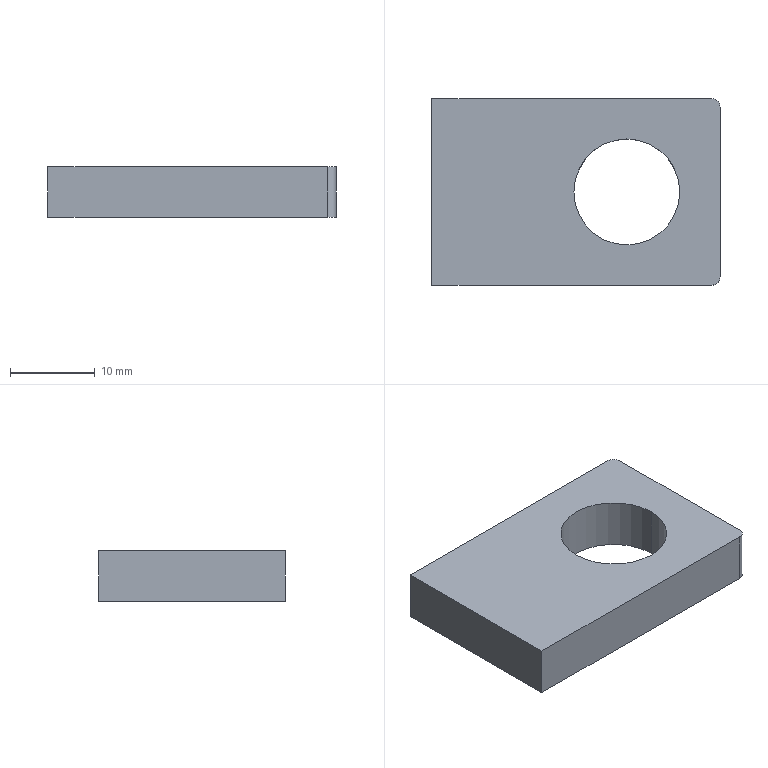Part | SolidWorks | features FlatPattern 1, SMBaseFlange 1, SheetMetal 1 | 1 solid | 10 faces | box 34 x 22 x 6 mm | volume 3749 mm3 | plane 6 | cylinder 4 | commonest cylinder face diameters 2 x2 12.5 x2
STEP:
#1=CARTESIAN_POINT('',(-6.25,0.,6.));
#2=VERTEX_POINT('',#1);
#3=CARTESIAN_POINT('',(6.25,0.,6.));
#4=VERTEX_POINT('',#3);
#5=CARTESIAN_POINT('',(0.,0.,6.));
#6=DIRECTION('',(0.,0.,1.));
#7=DIRECTION('',(1.,0.,0.));
#8=AXIS2_PLACEMENT_3D('',#5,#6,#7);
#9=CIRCLE('',#8,6.25);
#10=EDGE_CURVE('',#2,#4,#9,.T.);
#11=ORIENTED_EDGE('',*,*,#10,.T.);
#12=CARTESIAN_POINT('',(6.25,0.,0.));
#13=VERTEX_POINT('',#12);
#14=CARTESIAN_POINT('',(6.25,0.,6.));
#15=DIRECTION('',(0.,0.,-1.));
#16=VECTOR('',#15,1000.);
#17=LINE('',#14,#16);
#18=EDGE_CURVE('',#4,#13,#17,.T.);
#19=ORIENTED_EDGE('',*,*,#18,.T.);
#20=CARTESIAN_POINT('',(-6.25,0.,0.));
#21=VERTEX_POINT('',#20);
#22=CARTESIAN_POINT('',(0.,0.,0.));
#23=DIRECTION('',(0.,0.,1.));
#24=DIRECTION('',(1.,0.,0.));
#25=AXIS2_PLACEMENT_3D('',#22,#23,#24);
#26=CIRCLE('',#25,6.25);
#27=EDGE_CURVE('',#21,#13,#26,.T.);
#28=ORIENTED_EDGE('',*,*,#27,.F.);
#29=CARTESIAN_POINT('',(-6.25,0.,6.));
#30=DIRECTION('',(0.,0.,-1.));
#31=VECTOR('',#30,1000.);
#32=LINE('',#29,#31);
#33=EDGE_CURVE('',#2,#21,#32,.T.);
#34=ORIENTED_EDGE('',*,*,#33,.F.);
#35=EDGE_LOOP('',(#11,#19,#28,#34));
#36=FACE_OUTER_BOUND('',#35,.T.);
#37=CARTESIAN_POINT('',(0.,0.,6.));
#38=DIRECTION('',(0.,0.,-1.));
#39=DIRECTION('',(-1.,0.,0.));
#40=AXIS2_PLACEMENT_3D('',#37,#38,#39);
#41=CYLINDRICAL_SURFACE('',#40,6.25);
#42=ADVANCED_FACE('',(#36),#41,.F.);
#43=CARTESIAN_POINT('',(-23.,11.,6.));
#44=VERTEX_POINT('',#43);
#45=CARTESIAN_POINT('',(-23.,-11.,6.));
#46=VERTEX_POINT('',#45);
#47=CARTESIAN_POINT('',(-23.,11.,6.));
#48=DIRECTION('',(0.,-1.,0.));
#49=VECTOR('',#48,1000.);
#50=LINE('',#47,#49);
#51=EDGE_CURVE('',#44,#46,#50,.T.);
#52=ORIENTED_EDGE('',*,*,#51,.T.);
#53=CARTESIAN_POINT('',(10.,-11.,6.));
#54=VERTEX_POINT('',#53);
#55=CARTESIAN_POINT('',(10.,-11.,6.));
#56=DIRECTION('',(1.,0.,0.));
#57=VECTOR('',#56,1000.);
#58=LINE('',#55,#57);
#59=EDGE_CURVE('',#46,#54,#58,.T.);
#60=ORIENTED_EDGE('',*,*,#59,.T.);
#61=CARTESIAN_POINT('',(11.,-10.,6.));
#62=VERTEX_POINT('',#61);
#63=CARTESIAN_POINT('',(10.,-10.,6.));
#64=DIRECTION('',(0.,0.,1.));
#65=DIRECTION('',(-1.,0.,0.));
#66=AXIS2_PLACEMENT_3D('',#63,#64,#65);
#67=CIRCLE('',#66,1.);
#68=EDGE_CURVE('',#54,#62,#67,.T.);
#69=ORIENTED_EDGE('',*,*,#68,.T.);
#70=CARTESIAN_POINT('',(11.,10.,6.));
#71=VERTEX_POINT('',#70);
#72=CARTESIAN_POINT('',(11.,10.,6.));
#73=DIRECTION('',(0.,1.,0.));
#74=VECTOR('',#73,1000.);
#75=LINE('',#72,#74);
#76=EDGE_CURVE('',#62,#71,#75,.T.);
#77=ORIENTED_EDGE('',*,*,#76,.T.);
#78=CARTESIAN_POINT('',(10.,11.,6.));
#79=VERTEX_POINT('',#78);
#80=CARTESIAN_POINT('',(10.,10.,6.));
#81=DIRECTION('',(0.,0.,1.));
#82=DIRECTION('',(-1.,0.,0.));
#83=AXIS2_PLACEMENT_3D('',#80,#81,#82);
#84=CIRCLE('',#83,1.);
#85=EDGE_CURVE('',#71,#79,#84,.T.);
#86=ORIENTED_EDGE('',*,*,#85,.T.);
#87=CARTESIAN_POINT('',(10.,11.,6.));
#88=DIRECTION('',(-1.,0.,0.));
#89=VECTOR('',#88,1000.);
#90=LINE('',#87,#89);
#91=EDGE_CURVE('',#79,#44,#90,.T.);
#92=ORIENTED_EDGE('',*,*,#91,.T.);
#93=EDGE_LOOP('',(#52,#60,#69,#77,#86,#92));
#94=FACE_OUTER_BOUND('',#93,.T.);
#95=ORIENTED_EDGE('',*,*,#10,.F.);
#96=CARTESIAN_POINT('',(0.,0.,6.));
#97=DIRECTION('',(0.,0.,1.));
#98=DIRECTION('',(1.,0.,0.));
#99=AXIS2_PLACEMENT_3D('',#96,#97,#98);
#100=CIRCLE('',#99,6.25);
#101=EDGE_CURVE('',#4,#2,#100,.T.);
#102=ORIENTED_EDGE('',*,*,#101,.F.);
#103=EDGE_LOOP('',(#95,#102));
#104=FACE_BOUND('',#103,.T.);
#105=CARTESIAN_POINT('',(10.,-10.,6.));
#106=DIRECTION('',(0.,0.,-1.));
#107=DIRECTION('',(-1.,0.,0.));
#108=AXIS2_PLACEMENT_3D('',#105,#106,#107);
#109=PLANE('',#108);
#110=ADVANCED_FACE('',(#94,#104),#109,.F.);
#111=CARTESIAN_POINT('',(-23.,11.,0.));
#112=VERTEX_POINT('',#111);
#113=CARTESIAN_POINT('',(-23.,-11.,0.));
#114=VERTEX_POINT('',#113);
#115=CARTESIAN_POINT('',(-23.,11.,0.));
#116=DIRECTION('',(0.,-1.,0.));
#117=VECTOR('',#116,1000.);
#118=LINE('',#115,#117);
#119=EDGE_CURVE('',#112,#114,#118,.T.);
#120=ORIENTED_EDGE('',*,*,#119,.F.);
#121=CARTESIAN_POINT('',(10.,11.,0.));
#122=VERTEX_POINT('',#121);
#123=CARTESIAN_POINT('',(10.,11.,0.));
#124=DIRECTION('',(-1.,0.,0.));
#125=VECTOR('',#124,1000.);
#126=LINE('',#123,#125);
#127=EDGE_CURVE('',#122,#112,#126,.T.);
#128=ORIENTED_EDGE('',*,*,#127,.F.);
#129=CARTESIAN_POINT('',(11.,10.,0.));
#130=VERTEX_POINT('',#129);
#131=CARTESIAN_POINT('',(10.,10.,0.));
#132=DIRECTION('',(0.,0.,1.));
#133=DIRECTION('',(-1.,0.,0.));
#134=AXIS2_PLACEMENT_3D('',#131,#132,#133);
#135=CIRCLE('',#134,1.);
#136=EDGE_CURVE('',#130,#122,#135,.T.);
#137=ORIENTED_EDGE('',*,*,#136,.F.);
#138=CARTESIAN_POINT('',(11.,-10.,0.));
#139=VERTEX_POINT('',#138);
#140=CARTESIAN_POINT('',(11.,10.,0.));
#141=DIRECTION('',(0.,1.,0.));
#142=VECTOR('',#141,1000.);
#143=LINE('',#140,#142);
#144=EDGE_CURVE('',#139,#130,#143,.T.);
#145=ORIENTED_EDGE('',*,*,#144,.F.);
#146=CARTESIAN_POINT('',(10.,-11.,0.));
#147=VERTEX_POINT('',#146);
#148=CARTESIAN_POINT('',(10.,-10.,0.));
#149=DIRECTION('',(0.,0.,1.));
#150=DIRECTION('',(-1.,0.,0.));
#151=AXIS2_PLACEMENT_3D('',#148,#149,#150);
#152=CIRCLE('',#151,1.);
#153=EDGE_CURVE('',#147,#139,#152,.T.);
#154=ORIENTED_EDGE('',*,*,#153,.F.);
#155=CARTESIAN_POINT('',(10.,-11.,0.));
#156=DIRECTION('',(1.,0.,0.));
#157=VECTOR('',#156,1000.);
#158=LINE('',#155,#157);
#159=EDGE_CURVE('',#114,#147,#158,.T.);
#160=ORIENTED_EDGE('',*,*,#159,.F.);
#161=EDGE_LOOP('',(#120,#128,#137,#145,#154,#160));
#162=FACE_OUTER_BOUND('',#161,.T.);
#163=ORIENTED_EDGE('',*,*,#27,.T.);
#164=CARTESIAN_POINT('',(0.,0.,0.));
#165=DIRECTION('',(0.,0.,1.));
#166=DIRECTION('',(1.,0.,0.));
#167=AXIS2_PLACEMENT_3D('',#164,#165,#166);
#168=CIRCLE('',#167,6.25);
#169=EDGE_CURVE('',#13,#21,#168,.T.);
#170=ORIENTED_EDGE('',*,*,#169,.T.);
#171=EDGE_LOOP('',(#163,#170));
#172=FACE_BOUND('',#171,.T.);
#173=CARTESIAN_POINT('',(10.,-10.,0.));
#174=DIRECTION('',(0.,0.,-1.));
#175=DIRECTION('',(-1.,0.,0.));
#176=AXIS2_PLACEMENT_3D('',#173,#174,#175);
#177=PLANE('',#176);
#178=ADVANCED_FACE('',(#162,#172),#177,.T.);
#179=ORIENTED_EDGE('',*,*,#119,.T.);
#180=CARTESIAN_POINT('',(-23.,-11.,6.));
#181=DIRECTION('',(0.,0.,-1.));
#182=VECTOR('',#181,1000.);
#183=LINE('',#180,#182);
#184=EDGE_CURVE('',#46,#114,#183,.T.);
#185=ORIENTED_EDGE('',*,*,#184,.F.);
#186=ORIENTED_EDGE('',*,*,#51,.F.);
#187=CARTESIAN_POINT('',(-23.,11.,6.));
#188=DIRECTION('',(0.,0.,-1.));
#189=VECTOR('',#188,1000.);
#190=LINE('',#187,#189);
#191=EDGE_CURVE('',#44,#112,#190,.T.);
#192=ORIENTED_EDGE('',*,*,#191,.T.);
#193=EDGE_LOOP('',(#179,#185,#186,#192));
#194=FACE_OUTER_BOUND('',#193,.T.);
#195=CARTESIAN_POINT('',(-23.,11.,6.));
#196=DIRECTION('',(1.,0.,0.));
#197=DIRECTION('',(0.,1.,0.));
#198=AXIS2_PLACEMENT_3D('',#195,#196,#197);
#199=PLANE('',#198);
#200=ADVANCED_FACE('',(#194),#199,.F.);
#201=ORIENTED_EDGE('',*,*,#159,.T.);
#202=CARTESIAN_POINT('',(10.,-11.,6.));
#203=DIRECTION('',(0.,0.,-1.));
#204=VECTOR('',#203,1000.);
#205=LINE('',#202,#204);
#206=EDGE_CURVE('',#54,#147,#205,.T.);
#207=ORIENTED_EDGE('',*,*,#206,.F.);
#208=ORIENTED_EDGE('',*,*,#59,.F.);
#209=ORIENTED_EDGE('',*,*,#184,.T.);
#210=EDGE_LOOP('',(#201,#207,#208,#209));
#211=FACE_OUTER_BOUND('',#210,.T.);
#212=CARTESIAN_POINT('',(10.,-11.,6.));
#213=DIRECTION('',(0.,1.,0.));
#214=DIRECTION('',(-1.,0.,0.));
#215=AXIS2_PLACEMENT_3D('',#212,#213,#214);
#216=PLANE('',#215);
#217=ADVANCED_FACE('',(#211),#216,.F.);
#218=ORIENTED_EDGE('',*,*,#153,.T.);
#219=CARTESIAN_POINT('',(11.,-10.,6.));
#220=DIRECTION('',(0.,0.,-1.));
#221=VECTOR('',#220,1000.);
#222=LINE('',#219,#221);
#223=EDGE_CURVE('',#62,#139,#222,.T.);
#224=ORIENTED_EDGE('',*,*,#223,.F.);
#225=ORIENTED_EDGE('',*,*,#68,.F.);
#226=ORIENTED_EDGE('',*,*,#206,.T.);
#227=EDGE_LOOP('',(#218,#224,#225,#226));
#228=FACE_OUTER_BOUND('',#227,.T.);
#229=CARTESIAN_POINT('',(10.,-10.,6.));
#230=DIRECTION('',(0.,0.,-1.));
#231=DIRECTION('',(-1.,0.,0.));
#232=AXIS2_PLACEMENT_3D('',#229,#230,#231);
#233=CYLINDRICAL_SURFACE('',#232,1.);
#234=ADVANCED_FACE('',(#228),#233,.T.);
#235=ORIENTED_EDGE('',*,*,#144,.T.);
#236=CARTESIAN_POINT('',(11.,10.,6.));
#237=DIRECTION('',(0.,0.,-1.));
#238=VECTOR('',#237,1000.);
#239=LINE('',#236,#238);
#240=EDGE_CURVE('',#71,#130,#239,.T.);
#241=ORIENTED_EDGE('',*,*,#240,.F.);
#242=ORIENTED_EDGE('',*,*,#76,.F.);
#243=ORIENTED_EDGE('',*,*,#223,.T.);
#244=EDGE_LOOP('',(#235,#241,#242,#243));
#245=FACE_OUTER_BOUND('',#244,.T.);
#246=CARTESIAN_POINT('',(11.,10.,6.));
#247=DIRECTION('',(-1.,0.,0.));
#248=DIRECTION('',(0.,-1.,0.));
#249=AXIS2_PLACEMENT_3D('',#246,#247,#248);
#250=PLANE('',#249);
#251=ADVANCED_FACE('',(#245),#250,.F.);
#252=ORIENTED_EDGE('',*,*,#136,.T.);
#253=CARTESIAN_POINT('',(10.,11.,6.));
#254=DIRECTION('',(0.,0.,-1.));
#255=VECTOR('',#254,1000.);
#256=LINE('',#253,#255);
#257=EDGE_CURVE('',#79,#122,#256,.T.);
#258=ORIENTED_EDGE('',*,*,#257,.F.);
#259=ORIENTED_EDGE('',*,*,#85,.F.);
#260=ORIENTED_EDGE('',*,*,#240,.T.);
#261=EDGE_LOOP('',(#252,#258,#259,#260));
#262=FACE_OUTER_BOUND('',#261,.T.);
#263=CARTESIAN_POINT('',(10.,10.,6.));
#264=DIRECTION('',(0.,0.,-1.));
#265=DIRECTION('',(-1.,0.,0.));
#266=AXIS2_PLACEMENT_3D('',#263,#264,#265);
#267=CYLINDRICAL_SURFACE('',#266,1.);
#268=ADVANCED_FACE('',(#262),#267,.T.);
#269=ORIENTED_EDGE('',*,*,#127,.T.);
#270=ORIENTED_EDGE('',*,*,#191,.F.);
#271=ORIENTED_EDGE('',*,*,#91,.F.);
#272=ORIENTED_EDGE('',*,*,#257,.T.);
#273=EDGE_LOOP('',(#269,#270,#271,#272));
#274=FACE_OUTER_BOUND('',#273,.T.);
#275=CARTESIAN_POINT('',(10.,11.,6.));
#276=DIRECTION('',(0.,-1.,0.));
#277=DIRECTION('',(0.,0.,-1.));
#278=AXIS2_PLACEMENT_3D('',#275,#276,#277);
#279=PLANE('',#278);
#280=ADVANCED_FACE('',(#274),#279,.F.);
#281=ORIENTED_EDGE('',*,*,#18,.F.);
#282=ORIENTED_EDGE('',*,*,#101,.T.);
#283=ORIENTED_EDGE('',*,*,#33,.T.);
#284=ORIENTED_EDGE('',*,*,#169,.F.);
#285=EDGE_LOOP('',(#281,#282,#283,#284));
#286=FACE_OUTER_BOUND('',#285,.T.);
#287=CARTESIAN_POINT('',(0.,0.,6.));
#288=DIRECTION('',(0.,0.,-1.));
#289=DIRECTION('',(-1.,0.,0.));
#290=AXIS2_PLACEMENT_3D('',#287,#288,#289);
#291=CYLINDRICAL_SURFACE('',#290,6.25);
#292=ADVANCED_FACE('',(#286),#291,.F.);
#293=CLOSED_SHELL('',(#42,#110,#178,#200,#217,#234,#251,#268,#280,#292));
#294=MANIFOLD_SOLID_BREP('',#293);
#295=CARTESIAN_POINT('',(0.,0.,0.));
#296=DIRECTION('',(0.,0.,1.));
#297=DIRECTION('',(1.,0.,0.));
#298=AXIS2_PLACEMENT_3D('',#295,#296,#297);
#299=(LENGTH_UNIT()NAMED_UNIT(*)SI_UNIT(.MILLI.,.METRE.));
#300=UNCERTAINTY_MEASURE_WITH_UNIT(LENGTH_MEASURE(0.00001),#299,'','');
#301=(NAMED_UNIT(*)PLANE_ANGLE_UNIT()SI_UNIT($,.RADIAN.));
#302=(NAMED_UNIT(*)SI_UNIT($,.STERADIAN.)SOLID_ANGLE_UNIT());
#303=(GEOMETRIC_REPRESENTATION_CONTEXT(3)GLOBAL_UNCERTAINTY_ASSIGNED_CONTEXT((#300))GLOBAL_UNIT_ASSIGNED_CONTEXT((#299,#301,#302))REPRESENTATION_CONTEXT('',''));
#304=ADVANCED_BREP_SHAPE_REPRESENTATION('',(#294,#298),#303);